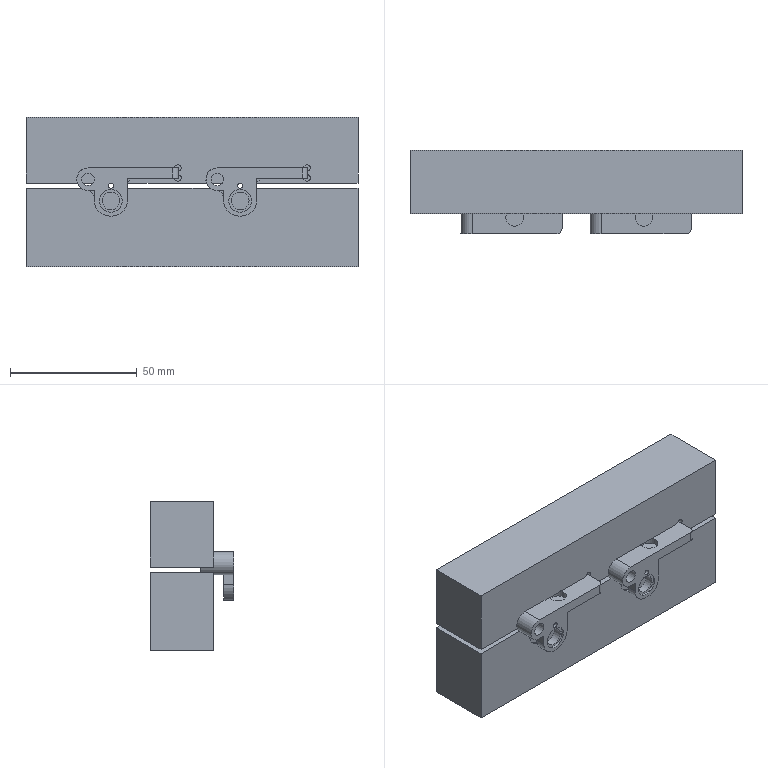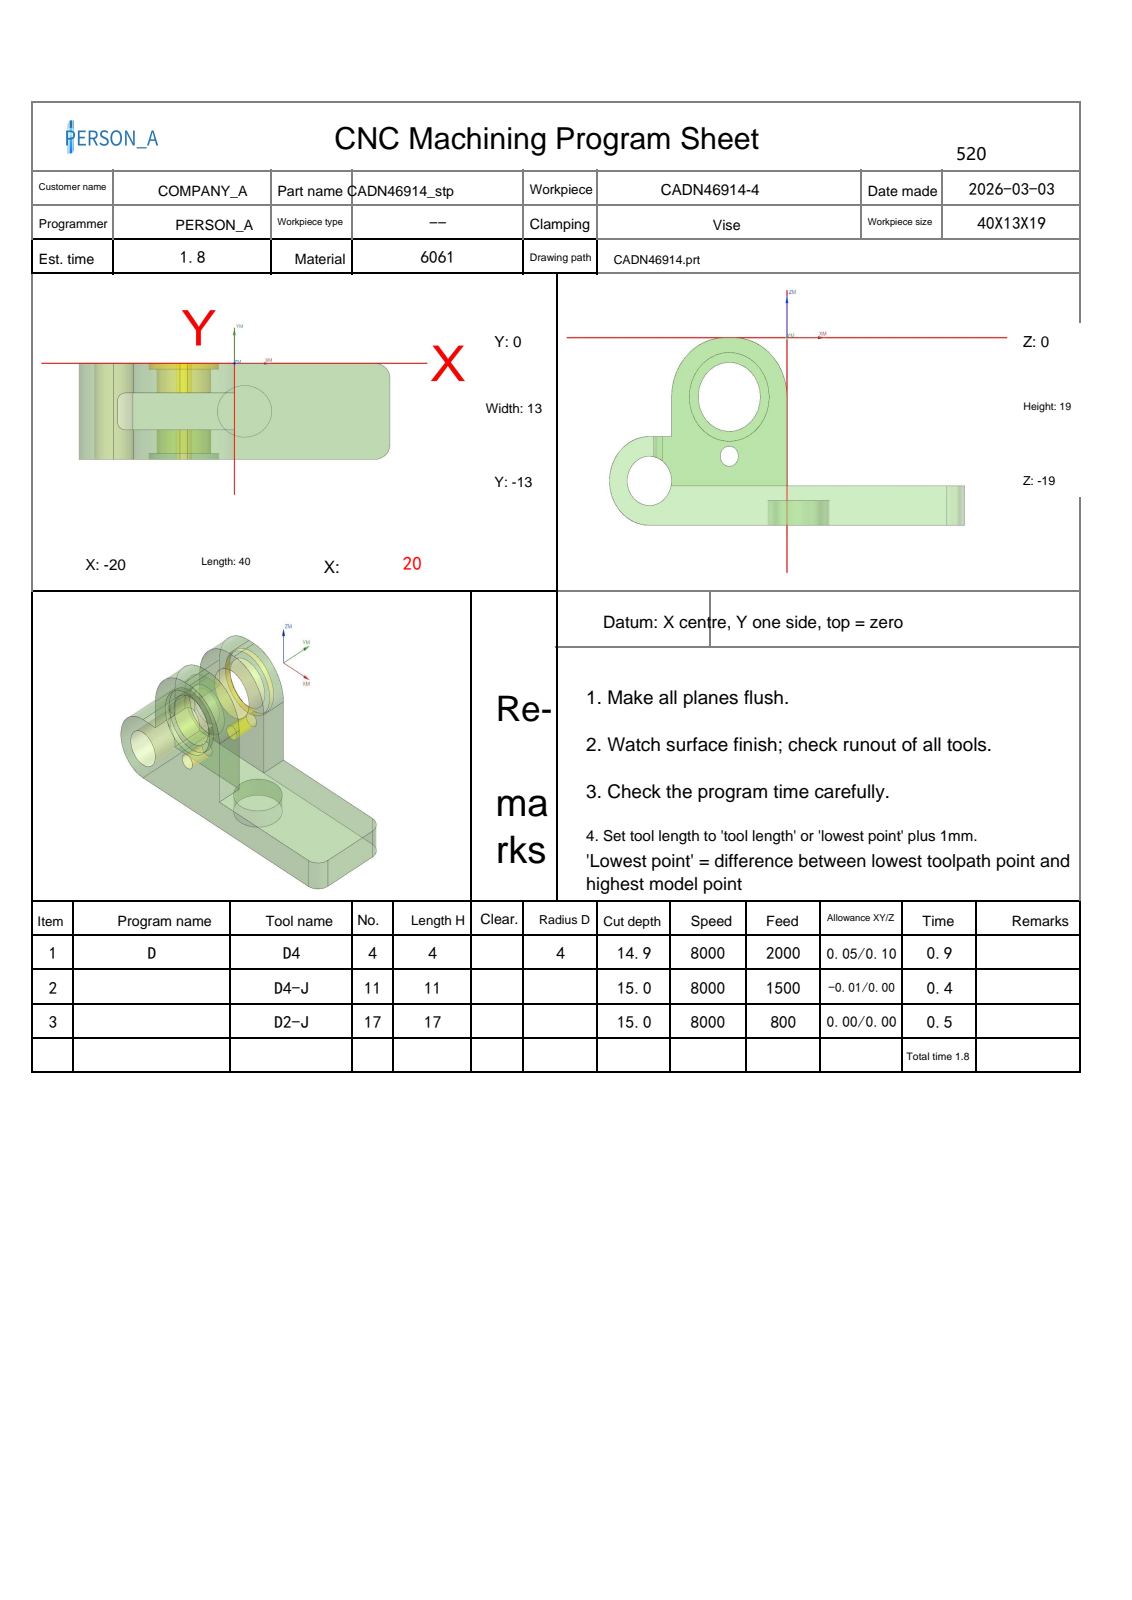NC program | NX | posted by the shop | part box 131 x 33 x 59 mm
Lines 813 to 1839 of 3020:
N3 T17 M06
(D2-J  D=2. R=0. H=17 ce=0.00 di=0.00)
G00 G90 G54 X-12.651 Y-5.2 M03 S8000
G43 H17 Z50.
M08
Z-9.9
G01 X-12.652 Y-5.198 Z-9.93 F800.
X-12.653 Y-5.191 Z-9.958
X-12.656 Y-5.18 Z-9.982
X-12.661 Y-5.165 Z-10.004
X-12.667 Y-5.149 Z-10.023
X-12.675 Y-5.13 Z-10.04
X-12.685 Y-5.11 Z-10.054
X-12.697 Y-5.09 Z-10.066
X-12.711 Y-5.071 Z-10.076
X-12.728 Y-5.052 Z-10.084
X-12.747 Y-5.035 Z-10.09
X-12.769 Y-5.021 Z-10.095
X-12.793 Y-5.01 Z-10.098
X-12.821 Y-5.003 Z-10.099
X-12.851 Y-5. Z-10.1
X-14.
Y-6.149
X-13.989 Y-6.178
X-13.958 Y-6.19
X-13.91 Y-6.188
X-13.849 Y-6.174
X-13.777 Y-6.147 Z-10.101
X-13.699 Y-6.111 Z-10.102
X-13.616 Y-6.067 Z-10.105
X-13.534 Y-6.017 Z-10.108
X-13.325 Y-5.859 Z-10.122
X-13.141 Y-5.673 Z-10.141
X-12.984 Y-5.464 Z-10.162
X-12.934 Y-5.381 Z-10.17
X-12.89 Y-5.299 Z-10.177
X-12.854 Y-5.221 Z-10.183
X-12.827 Y-5.15 Z-10.189
X-12.812 Y-5.089 Z-10.193
X-12.81 Y-5.042 Z-10.197
X-12.822 Y-5.011 Z-10.199
X-12.851 Y-5. Z-10.2
X-13.99
X-14.
Y-6.149
X-13.989 Y-6.178 Z-10.201
X-13.959 Y-6.19 Z-10.202
X-13.911 Y-6.187 Z-10.205
X-13.851 Y-6.172 Z-10.208
X-13.78 Y-6.145 Z-10.212
X-13.703 Y-6.108 Z-10.217
X-13.621 Y-6.064 Z-10.222
X-13.539 Y-6.013 Z-10.227
X-13.331 Y-5.855 Z-10.242
X-13.145 Y-5.669 Z-10.258
X-12.987 Y-5.461 Z-10.273
X-12.936 Y-5.379 Z-10.278
X-12.892 Y-5.298 Z-10.283
X-12.855 Y-5.22 Z-10.288
X-12.828 Y-5.149 Z-10.292
X-12.813 Y-5.089 Z-10.295
X-12.81 Y-5.041 Z-10.298
X-12.822 Y-5.011 Z-10.299
X-12.851 Y-5. Z-10.3
X-13.99
X-14.
Y-6.149
X-13.989 Y-6.178 Z-10.301
X-13.959 Y-6.19 Z-10.302
X-13.911 Y-6.187 Z-10.305
X-13.851 Y-6.172 Z-10.308
X-13.78 Y-6.145 Z-10.312
X-13.703 Y-6.108 Z-10.317
X-13.621 Y-6.064 Z-10.322
X-13.539 Y-6.013 Z-10.327
X-13.331 Y-5.855 Z-10.342
X-13.145 Y-5.669 Z-10.358
X-12.987 Y-5.461 Z-10.373
X-12.936 Y-5.379 Z-10.378
X-12.892 Y-5.298 Z-10.383
X-12.855 Y-5.22 Z-10.388
X-12.828 Y-5.149 Z-10.392
X-12.813 Y-5.089 Z-10.395
X-12.81 Y-5.041 Z-10.398
X-12.822 Y-5.011 Z-10.399
X-12.851 Y-5. Z-10.4
X-13.99
X-14.
Y-6.149
X-13.989 Y-6.178 Z-10.401
X-13.959 Y-6.19 Z-10.402
X-13.911 Y-6.187 Z-10.405
X-13.851 Y-6.172 Z-10.408
X-13.78 Y-6.145 Z-10.412
X-13.703 Y-6.108 Z-10.417
X-13.621 Y-6.064 Z-10.422
X-13.539 Y-6.013 Z-10.427
X-13.331 Y-5.855 Z-10.442
X-13.145 Y-5.669 Z-10.458
X-12.987 Y-5.461 Z-10.473
X-12.936 Y-5.379 Z-10.478
X-12.892 Y-5.298 Z-10.483
X-12.855 Y-5.22 Z-10.488
X-12.828 Y-5.149 Z-10.492
X-12.813 Y-5.089 Z-10.495
X-12.81 Y-5.041 Z-10.498
X-12.822 Y-5.011 Z-10.499
X-12.851 Y-5. Z-10.5
X-13.99
X-14.
Y-6.149
X-13.989 Y-6.178 Z-10.501
X-13.959 Y-6.19 Z-10.502
X-13.911 Y-6.187 Z-10.505
X-13.851 Y-6.172 Z-10.508
X-13.78 Y-6.145 Z-10.512
X-13.703 Y-6.108 Z-10.517
X-13.621 Y-6.064 Z-10.522
X-13.539 Y-6.013 Z-10.527
X-13.331 Y-5.855 Z-10.542
X-13.145 Y-5.669 Z-10.558
X-12.987 Y-5.461 Z-10.573
X-12.936 Y-5.379 Z-10.578
X-12.892 Y-5.298 Z-10.583
X-12.855 Y-5.22 Z-10.588
X-12.828 Y-5.149 Z-10.592
X-12.813 Y-5.089 Z-10.595
X-12.81 Y-5.041 Z-10.598
X-12.822 Y-5.011 Z-10.599
X-12.851 Y-5. Z-10.6
X-13.99
X-14.
Y-6.149
X-13.989 Y-6.178 Z-10.601
X-13.959 Y-6.19 Z-10.602
X-13.911 Y-6.187 Z-10.605
X-13.851 Y-6.172 Z-10.608
X-13.78 Y-6.145 Z-10.612
X-13.703 Y-6.108 Z-10.617
X-13.621 Y-6.064 Z-10.622
X-13.539 Y-6.013 Z-10.627
X-13.331 Y-5.855 Z-10.642
X-13.145 Y-5.669 Z-10.658
X-12.987 Y-5.461 Z-10.673
X-12.936 Y-5.379 Z-10.678
X-12.892 Y-5.298 Z-10.683
X-12.855 Y-5.22 Z-10.688
X-12.828 Y-5.149 Z-10.692
X-12.813 Y-5.089 Z-10.695
X-12.81 Y-5.041 Z-10.698
X-12.822 Y-5.011 Z-10.699
X-12.851 Y-5. Z-10.7
X-13.99
X-14.
Y-6.149
X-13.989 Y-6.178 Z-10.701
X-13.959 Y-6.19 Z-10.702
X-13.911 Y-6.187 Z-10.705
X-13.851 Y-6.172 Z-10.708
X-13.78 Y-6.145 Z-10.712
X-13.703 Y-6.108 Z-10.717
X-13.621 Y-6.064 Z-10.722
X-13.539 Y-6.013 Z-10.727
X-13.331 Y-5.855 Z-10.742
X-13.145 Y-5.669 Z-10.758
X-12.987 Y-5.461 Z-10.773
X-12.936 Y-5.379 Z-10.778
X-12.892 Y-5.298 Z-10.783
X-12.855 Y-5.22 Z-10.788
X-12.828 Y-5.149 Z-10.792
X-12.813 Y-5.089 Z-10.795
X-12.81 Y-5.041 Z-10.798
X-12.822 Y-5.011 Z-10.799
X-12.851 Y-5. Z-10.8
X-13.99
X-14.
Y-6.149
X-13.989 Y-6.178 Z-10.801
X-13.959 Y-6.19 Z-10.802
X-13.911 Y-6.187 Z-10.805
X-13.851 Y-6.172 Z-10.808
X-13.78 Y-6.145 Z-10.812
X-13.703 Y-6.108 Z-10.817
X-13.621 Y-6.064 Z-10.822
X-13.539 Y-6.013 Z-10.827
X-13.331 Y-5.855 Z-10.842
X-13.145 Y-5.669 Z-10.858
X-12.987 Y-5.461 Z-10.873
X-12.936 Y-5.379 Z-10.878
X-12.892 Y-5.298 Z-10.883
X-12.855 Y-5.22 Z-10.888
X-12.828 Y-5.149 Z-10.892
X-12.813 Y-5.089 Z-10.895
X-12.81 Y-5.041 Z-10.898
X-12.822 Y-5.011 Z-10.899
X-12.851 Y-5. Z-10.9
X-13.99
X-14.
Y-6.149
X-13.989 Y-6.178 Z-10.901
X-13.959 Y-6.19 Z-10.902
X-13.911 Y-6.187 Z-10.905
X-13.851 Y-6.172 Z-10.908
X-13.78 Y-6.145 Z-10.912
X-13.703 Y-6.108 Z-10.917
X-13.621 Y-6.064 Z-10.922
X-13.539 Y-6.013 Z-10.927
X-13.331 Y-5.855 Z-10.942
X-13.145 Y-5.669 Z-10.958
X-12.987 Y-5.461 Z-10.973
X-12.936 Y-5.379 Z-10.978
X-12.892 Y-5.298 Z-10.983
X-12.855 Y-5.22 Z-10.988
X-12.828 Y-5.149 Z-10.992
X-12.813 Y-5.089 Z-10.995
X-12.81 Y-5.041 Z-10.998
X-12.822 Y-5.011 Z-10.999
X-12.851 Y-5. Z-11.
X-13.99
X-14.
Y-6.149
X-13.989 Y-6.178 Z-11.001
X-13.959 Y-6.19 Z-11.002
X-13.911 Y-6.187 Z-11.005
X-13.851 Y-6.172 Z-11.008
X-13.78 Y-6.145 Z-11.012
X-13.703 Y-6.108 Z-11.017
X-13.621 Y-6.064 Z-11.022
X-13.539 Y-6.013 Z-11.027
X-13.331 Y-5.855 Z-11.042
X-13.145 Y-5.669 Z-11.058
X-12.987 Y-5.461 Z-11.073
X-12.936 Y-5.379 Z-11.078
X-12.892 Y-5.298 Z-11.083
X-12.855 Y-5.22 Z-11.088
X-12.828 Y-5.149 Z-11.092
X-12.813 Y-5.089 Z-11.095
X-12.81 Y-5.041 Z-11.098
X-12.822 Y-5.011 Z-11.099
X-12.851 Y-5. Z-11.1
X-13.99
X-14.
Y-6.149
X-13.989 Y-6.178 Z-11.101
X-13.959 Y-6.19 Z-11.102
X-13.911 Y-6.187 Z-11.105
X-13.851 Y-6.172 Z-11.108
X-13.78 Y-6.145 Z-11.112
X-13.703 Y-6.108 Z-11.117
X-13.621 Y-6.064 Z-11.122
X-13.539 Y-6.013 Z-11.127
X-13.331 Y-5.855 Z-11.142
X-13.145 Y-5.669 Z-11.158
X-12.987 Y-5.461 Z-11.173
X-12.936 Y-5.379 Z-11.178
X-12.892 Y-5.298 Z-11.183
X-12.855 Y-5.22 Z-11.188
X-12.828 Y-5.149 Z-11.192
X-12.813 Y-5.089 Z-11.195
X-12.81 Y-5.041 Z-11.198
X-12.822 Y-5.011 Z-11.199
X-12.851 Y-5. Z-11.2
X-13.99
X-14.
Y-6.149
X-13.989 Y-6.178 Z-11.201
X-13.959 Y-6.19 Z-11.202
X-13.911 Y-6.187 Z-11.205
X-13.851 Y-6.172 Z-11.208
X-13.78 Y-6.145 Z-11.212
X-13.703 Y-6.108 Z-11.217
X-13.621 Y-6.064 Z-11.222
X-13.539 Y-6.013 Z-11.227
X-13.331 Y-5.855 Z-11.242
X-13.145 Y-5.669 Z-11.258
X-12.987 Y-5.461 Z-11.273
X-12.936 Y-5.379 Z-11.278
X-12.892 Y-5.298 Z-11.283
X-12.855 Y-5.22 Z-11.288
X-12.828 Y-5.149 Z-11.292
X-12.813 Y-5.089 Z-11.295
X-12.81 Y-5.041 Z-11.298
X-12.822 Y-5.011 Z-11.299
X-12.851 Y-5. Z-11.3
X-13.99
X-14.
Y-6.149
X-13.989 Y-6.178 Z-11.301
X-13.959 Y-6.19 Z-11.302
X-13.911 Y-6.187 Z-11.305
X-13.851 Y-6.172 Z-11.308
X-13.78 Y-6.145 Z-11.312
X-13.703 Y-6.108 Z-11.317
X-13.621 Y-6.064 Z-11.322
X-13.539 Y-6.013 Z-11.327
X-13.331 Y-5.855 Z-11.342
X-13.145 Y-5.669 Z-11.358
X-12.987 Y-5.461 Z-11.373
X-12.936 Y-5.379 Z-11.378
X-12.892 Y-5.298 Z-11.383
X-12.855 Y-5.22 Z-11.388
X-12.828 Y-5.149 Z-11.392
X-12.813 Y-5.089 Z-11.395
X-12.81 Y-5.041 Z-11.398
X-12.822 Y-5.011 Z-11.399
X-12.851 Y-5. Z-11.4
X-13.99
X-14.
Y-6.149
X-13.989 Y-6.178 Z-11.401
X-13.959 Y-6.19 Z-11.402
X-13.911 Y-6.187 Z-11.405
X-13.851 Y-6.172 Z-11.408
X-13.78 Y-6.145 Z-11.412
X-13.703 Y-6.108 Z-11.417
X-13.621 Y-6.064 Z-11.422
X-13.539 Y-6.013 Z-11.427
X-13.331 Y-5.855 Z-11.442
X-13.145 Y-5.669 Z-11.458
X-12.987 Y-5.461 Z-11.473
X-12.936 Y-5.379 Z-11.478
X-12.892 Y-5.298 Z-11.483
X-12.855 Y-5.22 Z-11.488
X-12.828 Y-5.149 Z-11.492
X-12.813 Y-5.089 Z-11.495
X-12.81 Y-5.041 Z-11.498
X-12.822 Y-5.011 Z-11.499
X-12.851 Y-5. Z-11.5
X-13.99
X-14.
Y-6.149
X-13.989 Y-6.178 Z-11.501
X-13.959 Y-6.19 Z-11.502
X-13.911 Y-6.187 Z-11.505
X-13.851 Y-6.172 Z-11.508
X-13.78 Y-6.145 Z-11.512
X-13.703 Y-6.108 Z-11.517
X-13.621 Y-6.064 Z-11.522
X-13.539 Y-6.013 Z-11.527
X-13.331 Y-5.855 Z-11.542
X-13.145 Y-5.669 Z-11.558
X-12.987 Y-5.461 Z-11.573
X-12.936 Y-5.379 Z-11.578
X-12.892 Y-5.298 Z-11.583
X-12.855 Y-5.22 Z-11.588
X-12.828 Y-5.149 Z-11.592
X-12.813 Y-5.089 Z-11.595
X-12.81 Y-5.041 Z-11.598
X-12.822 Y-5.011 Z-11.599
X-12.851 Y-5. Z-11.6
X-13.99
X-14.
Y-6.149
X-13.989 Y-6.178 Z-11.601
X-13.959 Y-6.19 Z-11.602
X-13.911 Y-6.187 Z-11.605
X-13.851 Y-6.172 Z-11.608
X-13.78 Y-6.145 Z-11.612
X-13.703 Y-6.108 Z-11.617
X-13.621 Y-6.064 Z-11.622
X-13.539 Y-6.013 Z-11.627
X-13.331 Y-5.855 Z-11.642
X-13.145 Y-5.669 Z-11.658
X-12.987 Y-5.461 Z-11.673
X-12.936 Y-5.379 Z-11.678
X-12.892 Y-5.298 Z-11.683
X-12.855 Y-5.22 Z-11.688
X-12.828 Y-5.149 Z-11.692
X-12.813 Y-5.089 Z-11.695
X-12.81 Y-5.041 Z-11.698
X-12.822 Y-5.011 Z-11.699
X-12.851 Y-5. Z-11.7
X-13.99
X-14.
Y-6.149
X-13.989 Y-6.178 Z-11.701
X-13.959 Y-6.19 Z-11.702
X-13.911 Y-6.187 Z-11.705
X-13.851 Y-6.172 Z-11.708
X-13.78 Y-6.145 Z-11.712
X-13.703 Y-6.108 Z-11.717
X-13.621 Y-6.064 Z-11.722
X-13.539 Y-6.013 Z-11.727
X-13.331 Y-5.855 Z-11.742
X-13.145 Y-5.669 Z-11.758
X-12.987 Y-5.461 Z-11.773
X-12.936 Y-5.379 Z-11.778
X-12.892 Y-5.298 Z-11.783
X-12.855 Y-5.22 Z-11.788
X-12.828 Y-5.149 Z-11.792
X-12.813 Y-5.089 Z-11.795
X-12.81 Y-5.041 Z-11.798
X-12.822 Y-5.011 Z-11.799
X-12.851 Y-5. Z-11.8
X-13.99
X-14.
Y-6.149
X-13.989 Y-6.178 Z-11.801
X-13.959 Y-6.19 Z-11.802
X-13.911 Y-6.187 Z-11.805
X-13.851 Y-6.172 Z-11.808
X-13.78 Y-6.145 Z-11.812
X-13.703 Y-6.108 Z-11.817
X-13.621 Y-6.064 Z-11.822
X-13.539 Y-6.013 Z-11.827
X-13.331 Y-5.855 Z-11.842
X-13.145 Y-5.669 Z-11.858
X-12.987 Y-5.461 Z-11.873
X-12.936 Y-5.379 Z-11.878
X-12.892 Y-5.298 Z-11.883
X-12.855 Y-5.22 Z-11.888
X-12.828 Y-5.149 Z-11.892
X-12.813 Y-5.089 Z-11.895
X-12.81 Y-5.041 Z-11.898
X-12.822 Y-5.011 Z-11.899
X-12.851 Y-5. Z-11.9
X-13.99
X-14.
Y-6.149
X-13.989 Y-6.178 Z-11.901
X-13.959 Y-6.19 Z-11.902
X-13.911 Y-6.187 Z-11.905
X-13.851 Y-6.172 Z-11.908
X-13.78 Y-6.145 Z-11.912
X-13.703 Y-6.108 Z-11.917
X-13.621 Y-6.064 Z-11.922
X-13.539 Y-6.013 Z-11.927
X-13.331 Y-5.855 Z-11.942
X-13.145 Y-5.669 Z-11.958
X-12.987 Y-5.461 Z-11.973
X-12.936 Y-5.379 Z-11.978
X-12.892 Y-5.298 Z-11.983
X-12.855 Y-5.22 Z-11.988
X-12.828 Y-5.149 Z-11.992
X-12.813 Y-5.089 Z-11.995
X-12.81 Y-5.041 Z-11.998
X-12.822 Y-5.011 Z-11.999
X-12.851 Y-5. Z-12.
X-13.99
X-14.
Y-6.149
X-13.989 Y-6.178 Z-12.001
X-13.959 Y-6.19 Z-12.002
X-13.911 Y-6.187 Z-12.005
X-13.851 Y-6.172 Z-12.008
X-13.78 Y-6.145 Z-12.012
X-13.703 Y-6.108 Z-12.017
X-13.621 Y-6.064 Z-12.022
X-13.539 Y-6.013 Z-12.027
X-13.331 Y-5.855 Z-12.042
X-13.145 Y-5.669 Z-12.058
X-12.987 Y-5.461 Z-12.073
X-12.936 Y-5.379 Z-12.078
X-12.892 Y-5.298 Z-12.083
X-12.855 Y-5.22 Z-12.088
X-12.828 Y-5.149 Z-12.092
X-12.813 Y-5.089 Z-12.095
X-12.81 Y-5.041 Z-12.098
X-12.822 Y-5.011 Z-12.099
X-12.851 Y-5. Z-12.1
X-14.
Y-6.149
X-13.989 Y-6.179 Z-12.101
X-13.958 Y-6.194 Z-12.102
X-13.91 Y-6.196 Z-12.105
X-13.848 Y-6.186 Z-12.108
X-13.777 Y-6.165 Z-12.112
X-13.698 Y-6.134 Z-12.117
X-13.615 Y-6.094 Z-12.122
X-13.533 Y-6.046 Z-12.127
X-13.374 Y-5.933 Z-12.138
X-13.229 Y-5.798 Z-12.15
X-13.098 Y-5.646 Z-12.162
X-12.984 Y-5.48 Z-12.173
X-12.933 Y-5.394 Z-12.178
X-12.89 Y-5.309 Z-12.183
X-12.853 Y-5.228 Z-12.188
X-12.827 Y-5.155 Z-12.192
X-12.812 Y-5.092 Z-12.195
X-12.81 Y-5.043 Z-12.198
X-12.822 Y-5.011 Z-12.199
X-12.851 Y-5. Z-12.2
X-14.
Y-6.149
X-13.989 Y-6.18 Z-12.201
X-13.958 Y-6.197 Z-12.202
X-13.911 Y-6.202 Z-12.205
X-13.85 Y-6.195 Z-12.208
X-13.779 Y-6.177 Z-12.212
X-13.701 Y-6.15 Z-12.217
X-13.619 Y-6.113 Z-12.222
X-13.536 Y-6.068 Z-12.227
X-13.378 Y-5.956 Z-12.238
X-13.233 Y-5.819 Z-12.25
X-13.101 Y-5.663 Z-12.262
X-12.986 Y-5.492 Z-12.273
X-12.935 Y-5.404 Z-12.278
X-12.891 Y-5.317 Z-12.283
X-12.854 Y-5.234 Z-12.288
X-12.828 Y-5.158 Z-12.292
X-12.812 Y-5.094 Z-12.295
X-12.81 Y-5.044 Z-12.298
X-12.822 Y-5.012 Z-12.299
X-12.851 Y-5. Z-12.3
X-14.
Y-6.149
X-13.986 Y-6.184 Z-12.301
X-13.948 Y-6.202 Z-12.303
X-13.89 Y-6.206 Z-12.306
X-13.816 Y-6.195 Z-12.31
X-13.731 Y-6.171 Z-12.315
X-13.64 Y-6.134 Z-12.321
X-13.547 Y-6.085 Z-12.327
X-13.39 Y-5.974 Z-12.338
X-13.243 Y-5.836 Z-12.35
X-13.11 Y-5.676 Z-12.362
X-12.992 Y-5.502 Z-12.373
X-12.94 Y-5.412 Z-12.378
X-12.895 Y-5.323 Z-12.383
X-12.857 Y-5.238 Z-12.388
X-12.83 Y-5.161 Z-12.392
X-12.813 Y-5.096 Z-12.395
X-12.81 Y-5.045 Z-12.398
X-12.822 Y-5.012 Z-12.399
X-12.851 Y-5. Z-12.4
X-14.
Y-6.149
X-13.988 Y-6.184 Z-12.401
X-13.953 Y-6.203 Z-12.403
X-13.9 Y-6.208 Z-12.406
X-13.832 Y-6.198 Z-12.41
X-13.754 Y-6.175 Z-12.415
X-13.668 Y-6.139 Z-12.421
X-13.579 Y-6.091 Z-12.427
X-13.423 Y-5.981 Z-12.438
X-13.273 Y-5.842 Z-12.449
X-13.133 Y-5.681 Z-12.461
X-13.008 Y-5.506 Z-12.472
X-12.953 Y-5.415 Z-12.477
X-12.904 Y-5.325 Z-12.483
X-12.864 Y-5.24 Z-12.487
X-12.834 Y-5.162 Z-12.492
X-12.816 Y-5.096 Z-12.495
X-12.812 Y-5.045 Z-12.498
X-12.823 Y-5.012 Z-12.499
X-12.851 Y-5. Z-12.5
X-14.
Y-6.149
X-13.988 Y-6.184 Z-12.501
X-13.953 Y-6.203 Z-12.503
X-13.9 Y-6.208 Z-12.506
X-13.832 Y-6.199 Z-12.51
X-13.754 Y-6.176 Z-12.515
X-13.668 Y-6.14 Z-12.52
X-13.579 Y-6.092 Z-12.526
X-13.424 Y-5.982 Z-12.538
X-13.274 Y-5.843 Z-12.549
X-13.135 Y-5.682 Z-12.561
X-13.01 Y-5.506 Z-12.573
X-12.954 Y-5.415 Z-12.578
X-12.906 Y-5.325 Z-12.583
X-12.865 Y-5.24 Z-12.588
X-12.835 Y-5.162 Z-12.592
X-12.816 Y-5.096 Z-12.595
X-12.812 Y-5.045 Z-12.598
X-12.823 Y-5.012 Z-12.599
X-12.851 Y-5. Z-12.6
X-14.
Y-6.149
X-13.988 Y-6.184 Z-12.601
X-13.953 Y-6.203 Z-12.603
X-13.9 Y-6.208 Z-12.606
X-13.833 Y-6.198 Z-12.61
X-13.754 Y-6.175 Z-12.615
X-13.669 Y-6.139 Z-12.621
X-13.58 Y-6.092 Z-12.627
X-13.425 Y-5.981 Z-12.638
X-13.275 Y-5.842 Z-12.65
X-13.135 Y-5.682 Z-12.662
X-13.01 Y-5.506 Z-12.673
X-12.955 Y-5.415 Z-12.678
X-12.906 Y-5.325 Z-12.683
X-12.865 Y-5.24 Z-12.688
X-12.835 Y-5.162 Z-12.692
X-12.817 Y-5.096 Z-12.695
X-12.812 Y-5.045 Z-12.698
X-12.823 Y-5.012 Z-12.699
X-12.851 Y-5. Z-12.7
X-14.
Y-6.149
X-13.988 Y-6.184 Z-12.701
X-13.953 Y-6.203 Z-12.703
X-13.9 Y-6.208 Z-12.706
X-13.833 Y-6.198 Z-12.71
X-13.754 Y-6.175 Z-12.715
X-13.669 Y-6.139 Z-12.721
X-13.58 Y-6.092 Z-12.727
X-13.425 Y-5.981 Z-12.738
X-13.275 Y-5.842 Z-12.75
X-13.135 Y-5.682 Z-12.762
X-13.01 Y-5.506 Z-12.773
X-12.955 Y-5.415 Z-12.778
X-12.906 Y-5.325 Z-12.783
X-12.865 Y-5.24 Z-12.788
X-12.835 Y-5.162 Z-12.792
X-12.817 Y-5.096 Z-12.795
X-12.812 Y-5.045 Z-12.798
X-12.823 Y-5.012 Z-12.799
X-12.851 Y-5. Z-12.8
X-14.
Y-6.149
X-13.988 Y-6.184 Z-12.801
X-13.953 Y-6.203 Z-12.803
X-13.9 Y-6.208 Z-12.806
X-13.833 Y-6.198 Z-12.81
X-13.754 Y-6.175 Z-12.815
X-13.669 Y-6.139 Z-12.821
X-13.58 Y-6.092 Z-12.827
X-13.425 Y-5.981 Z-12.838
X-13.275 Y-5.842 Z-12.85
X-13.135 Y-5.682 Z-12.862
X-13.01 Y-5.506 Z-12.873
X-12.955 Y-5.415 Z-12.878
X-12.906 Y-5.325 Z-12.883
X-12.865 Y-5.24 Z-12.888
X-12.835 Y-5.162 Z-12.892
X-12.817 Y-5.096 Z-12.895
X-12.812 Y-5.045 Z-12.898
X-12.823 Y-5.012 Z-12.899
X-12.851 Y-5. Z-12.9
X-14.
Y-6.149
X-13.988 Y-6.184 Z-12.901
X-13.953 Y-6.203 Z-12.903
X-13.9 Y-6.208 Z-12.906
X-13.833 Y-6.198 Z-12.91
X-13.754 Y-6.175 Z-12.915
X-13.669 Y-6.139 Z-12.921
X-13.58 Y-6.092 Z-12.927
X-13.425 Y-5.981 Z-12.938
X-13.275 Y-5.842 Z-12.95
X-13.135 Y-5.682 Z-12.962
X-13.01 Y-5.506 Z-12.973
X-12.955 Y-5.415 Z-12.978
X-12.906 Y-5.325 Z-12.983
X-12.865 Y-5.24 Z-12.988
X-12.835 Y-5.162 Z-12.992
X-12.817 Y-5.096 Z-12.995
X-12.812 Y-5.045 Z-12.998
X-12.823 Y-5.012 Z-12.999
X-12.851 Y-5. Z-13.
X-14.
Y-6.149
X-13.988 Y-6.184 Z-13.001
X-13.953 Y-6.203 Z-13.003
X-13.9 Y-6.208 Z-13.006
X-13.833 Y-6.198 Z-13.01
X-13.754 Y-6.175 Z-13.015
X-13.669 Y-6.139 Z-13.021
X-13.58 Y-6.092 Z-13.027
X-13.425 Y-5.981 Z-13.038
X-13.275 Y-5.842 Z-13.05
X-13.135 Y-5.682 Z-13.062
X-13.01 Y-5.506 Z-13.073
X-12.955 Y-5.415 Z-13.078
X-12.906 Y-5.325 Z-13.083
X-12.865 Y-5.24 Z-13.088
X-12.835 Y-5.162 Z-13.092
X-12.817 Y-5.096 Z-13.095
X-12.812 Y-5.045 Z-13.098
X-12.823 Y-5.012 Z-13.099
X-12.851 Y-5. Z-13.1
X-14.
Y-6.149
X-13.988 Y-6.184 Z-13.101
X-13.953 Y-6.203 Z-13.103
X-13.9 Y-6.208 Z-13.106
X-13.833 Y-6.198 Z-13.11
X-13.754 Y-6.175 Z-13.115
X-13.669 Y-6.139 Z-13.121
X-13.58 Y-6.092 Z-13.127
X-13.425 Y-5.981 Z-13.138
X-13.275 Y-5.842 Z-13.15
X-13.135 Y-5.682 Z-13.162
X-13.01 Y-5.506 Z-13.173
X-12.955 Y-5.415 Z-13.178
X-12.906 Y-5.325 Z-13.183
X-12.865 Y-5.24 Z-13.188
X-12.835 Y-5.162 Z-13.192
X-12.817 Y-5.096 Z-13.195
X-12.812 Y-5.045 Z-13.198
X-12.823 Y-5.012 Z-13.199
X-12.851 Y-5. Z-13.2
X-14.
Y-6.149
X-13.988 Y-6.184 Z-13.201
X-13.953 Y-6.203 Z-13.203
X-13.9 Y-6.208 Z-13.206
X-13.833 Y-6.198 Z-13.21
X-13.754 Y-6.175 Z-13.215
X-13.669 Y-6.139 Z-13.221
X-13.58 Y-6.092 Z-13.227
X-13.425 Y-5.981 Z-13.238
X-13.275 Y-5.842 Z-13.25
X-13.135 Y-5.682 Z-13.262
X-13.01 Y-5.506 Z-13.273
X-12.955 Y-5.415 Z-13.278
X-12.906 Y-5.325 Z-13.283
X-12.865 Y-5.24 Z-13.288
X-12.835 Y-5.162 Z-13.292
X-12.817 Y-5.096 Z-13.295
X-12.812 Y-5.045 Z-13.298
X-12.823 Y-5.012 Z-13.299
X-12.851 Y-5. Z-13.3
X-14.
Y-6.149
X-13.988 Y-6.184 Z-13.301
X-13.953 Y-6.203 Z-13.303
X-13.9 Y-6.208 Z-13.306
X-13.833 Y-6.198 Z-13.31
X-13.754 Y-6.175 Z-13.315
X-13.669 Y-6.139 Z-13.321
X-13.58 Y-6.092 Z-13.327
X-13.425 Y-5.981 Z-13.338
X-13.275 Y-5.842 Z-13.35
X-13.135 Y-5.682 Z-13.362
X-13.01 Y-5.506 Z-13.373
X-12.955 Y-5.415 Z-13.378
X-12.906 Y-5.325 Z-13.383
X-12.865 Y-5.24 Z-13.388
X-12.835 Y-5.162 Z-13.392
X-12.817 Y-5.096 Z-13.395
X-12.812 Y-5.045 Z-13.398
X-12.823 Y-5.012 Z-13.399
X-12.851 Y-5. Z-13.4
X-14.
Y-6.149
X-13.988 Y-6.184 Z-13.401
X-13.953 Y-6.203 Z-13.403
X-13.9 Y-6.208 Z-13.406
X-13.833 Y-6.198 Z-13.41
X-13.754 Y-6.175 Z-13.415
X-13.669 Y-6.139 Z-13.421
X-13.58 Y-6.092 Z-13.427
X-13.425 Y-5.981 Z-13.438
X-13.275 Y-5.842 Z-13.45
X-13.135 Y-5.682 Z-13.462
X-13.01 Y-5.506 Z-13.473
X-12.955 Y-5.415 Z-13.478
X-12.906 Y-5.325 Z-13.483
X-12.865 Y-5.24 Z-13.488
X-12.835 Y-5.162 Z-13.492
X-12.817 Y-5.096 Z-13.495
X-12.812 Y-5.045 Z-13.498
X-12.823 Y-5.012 Z-13.499
X-12.851 Y-5. Z-13.5
X-14.
Y-6.149
X-13.988 Y-6.184 Z-13.501
X-13.953 Y-6.203 Z-13.503
X-13.9 Y-6.208 Z-13.506
X-13.833 Y-6.198 Z-13.51
X-13.754 Y-6.175 Z-13.515
X-13.669 Y-6.139 Z-13.521
X-13.58 Y-6.092 Z-13.527
X-13.425 Y-5.981 Z-13.538
X-13.275 Y-5.842 Z-13.55
X-13.135 Y-5.682 Z-13.562
X-13.01 Y-5.506 Z-13.573
X-12.955 Y-5.415 Z-13.578
X-12.906 Y-5.325 Z-13.583
X-12.865 Y-5.24 Z-13.588
X-12.835 Y-5.162 Z-13.592
X-12.817 Y-5.096 Z-13.595
X-12.812 Y-5.045 Z-13.598
X-12.823 Y-5.012 Z-13.599
X-12.851 Y-5. Z-13.6
X-14.
Y-6.149
X-13.988 Y-6.184 Z-13.601
X-13.953 Y-6.203 Z-13.603
X-13.9 Y-6.208 Z-13.606
X-13.833 Y-6.198 Z-13.61
X-13.754 Y-6.175 Z-13.615
X-13.669 Y-6.139 Z-13.621
X-13.58 Y-6.092 Z-13.627
X-13.425 Y-5.981 Z-13.638
X-13.275 Y-5.842 Z-13.65
X-13.135 Y-5.682 Z-13.662
X-13.01 Y-5.506 Z-13.673
X-12.955 Y-5.415 Z-13.678
X-12.906 Y-5.325 Z-13.683
X-12.865 Y-5.24 Z-13.688
X-12.835 Y-5.162 Z-13.692
X-12.817 Y-5.096 Z-13.695
X-12.812 Y-5.045 Z-13.698
X-12.823 Y-5.012 Z-13.699
X-12.851 Y-5. Z-13.7
X-14.
Y-6.149
X-13.988 Y-6.184 Z-13.701
X-13.953 Y-6.203 Z-13.703
X-13.9 Y-6.208 Z-13.706
X-13.833 Y-6.198 Z-13.71
X-13.754 Y-6.175 Z-13.715
X-13.669 Y-6.139 Z-13.721
X-13.58 Y-6.092 Z-13.727
X-13.425 Y-5.981 Z-13.738
X-13.275 Y-5.842 Z-13.75
X-13.135 Y-5.682 Z-13.762
X-13.01 Y-5.506 Z-13.773
X-12.955 Y-5.415 Z-13.778
X-12.906 Y-5.325 Z-13.783
X-12.865 Y-5.24 Z-13.788
X-12.835 Y-5.162 Z-13.792
X-12.817 Y-5.096 Z-13.795
X-12.812 Y-5.045 Z-13.798
X-12.823 Y-5.012 Z-13.799
X-12.851 Y-5. Z-13.8
X-14.
Y-6.149
X-13.988 Y-6.184 Z-13.801
X-13.953 Y-6.203 Z-13.803
X-13.9 Y-6.208 Z-13.806
X-13.833 Y-6.198 Z-13.81
X-13.754 Y-6.175 Z-13.815
X-13.669 Y-6.139 Z-13.821
X-13.58 Y-6.092 Z-13.827
X-13.425 Y-5.981 Z-13.838
X-13.275 Y-5.842 Z-13.85
X-13.135 Y-5.682 Z-13.862
X-13.01 Y-5.506 Z-13.873
X-12.955 Y-5.415 Z-13.878
X-12.906 Y-5.325 Z-13.883
X-12.865 Y-5.24 Z-13.888
X-12.835 Y-5.162 Z-13.892
X-12.817 Y-5.096 Z-13.895
X-12.812 Y-5.045 Z-13.898
X-12.823 Y-5.012 Z-13.899
X-12.851 Y-5. Z-13.9
X-14.
Y-6.149
X-13.988 Y-6.184 Z-13.901
X-13.953 Y-6.203 Z-13.903
X-13.9 Y-6.208 Z-13.906
X-13.833 Y-6.198 Z-13.91
X-13.754 Y-6.175 Z-13.915
X-13.669 Y-6.139 Z-13.921
X-13.58 Y-6.092 Z-13.927
X-13.425 Y-5.981 Z-13.938
X-13.275 Y-5.842 Z-13.95
X-13.135 Y-5.682 Z-13.962
X-13.01 Y-5.506 Z-13.973
X-12.955 Y-5.415 Z-13.978
X-12.906 Y-5.325 Z-13.983
X-12.865 Y-5.24 Z-13.988
X-12.835 Y-5.162 Z-13.992
X-12.817 Y-5.096 Z-13.995
X-12.812 Y-5.045 Z-13.998
X-12.823 Y-5.012 Z-13.999
X-12.851 Y-5. Z-14.
X-14.
Y-6.149
X-13.988 Y-6.184 Z-14.001
X-13.953 Y-6.203 Z-14.003
X-13.9 Y-6.208 Z-14.006
X-13.833 Y-6.198 Z-14.01
X-13.754 Y-6.175 Z-14.015
X-13.669 Y-6.139 Z-14.021
X-13.58 Y-6.092 Z-14.027
X-13.425 Y-5.981 Z-14.038
X-13.275 Y-5.842 Z-14.05
X-13.135 Y-5.682 Z-14.062
X-13.01 Y-5.506 Z-14.073
X-12.955 Y-5.415 Z-14.078
X-12.906 Y-5.325 Z-14.083
X-12.865 Y-5.24 Z-14.088
X-12.835 Y-5.162 Z-14.092
X-12.817 Y-5.096 Z-14.095
X-12.812 Y-5.045 Z-14.098
X-12.823 Y-5.012 Z-14.099
X-12.851 Y-5. Z-14.1
X-14.
Y-6.149
X-13.988 Y-6.184 Z-14.101
X-13.953 Y-6.203 Z-14.103
X-13.9 Y-6.208 Z-14.106
X-13.833 Y-6.198 Z-14.11
X-13.754 Y-6.175 Z-14.115
X-13.669 Y-6.139 Z-14.121
X-13.58 Y-6.092 Z-14.127
X-13.425 Y-5.981 Z-14.138
X-13.275 Y-5.842 Z-14.15
X-13.135 Y-5.682 Z-14.162
X-13.01 Y-5.506 Z-14.173
X-12.955 Y-5.415 Z-14.178
X-12.906 Y-5.325 Z-14.183
X-12.865 Y-5.24 Z-14.188
X-12.835 Y-5.162 Z-14.192
X-12.817 Y-5.096 Z-14.195
X-12.812 Y-5.045 Z-14.198
X-12.823 Y-5.012 Z-14.199
X-12.851 Y-5. Z-14.2
X-14.
Y-6.149
X-13.988 Y-6.184 Z-14.201
X-13.953 Y-6.203 Z-14.203
X-13.9 Y-6.208 Z-14.206
X-13.833 Y-6.198 Z-14.21
X-13.754 Y-6.175 Z-14.215
X-13.669 Y-6.139 Z-14.221
X-13.58 Y-6.092 Z-14.227
X-13.425 Y-5.981 Z-14.238
X-13.275 Y-5.842 Z-14.25
X-13.135 Y-5.682 Z-14.262
X-13.01 Y-5.506 Z-14.273
X-12.955 Y-5.415 Z-14.278
X-12.906 Y-5.325 Z-14.283
X-12.865 Y-5.24 Z-14.288
X-12.835 Y-5.162 Z-14.292
X-12.817 Y-5.096 Z-14.295
X-12.812 Y-5.045 Z-14.298
X-12.823 Y-5.012 Z-14.299
X-12.851 Y-5. Z-14.3
X-14.
Y-6.149
X-13.988 Y-6.184 Z-14.301
X-13.953 Y-6.203 Z-14.303
X-13.9 Y-6.208 Z-14.306
X-13.833 Y-6.198 Z-14.31
X-13.754 Y-6.175 Z-14.315
X-13.669 Y-6.139 Z-14.321
X-13.58 Y-6.092 Z-14.327
X-13.425 Y-5.981 Z-14.338
X-13.275 Y-5.842 Z-14.35
X-13.135 Y-5.682 Z-14.362
X-13.01 Y-5.506 Z-14.373
X-12.955 Y-5.415 Z-14.378
X-12.906 Y-5.325 Z-14.383
X-12.865 Y-5.24 Z-14.388
X-12.835 Y-5.162 Z-14.392
X-12.817 Y-5.096 Z-14.395
X-12.812 Y-5.045 Z-14.398
X-12.823 Y-5.012 Z-14.399
X-12.851 Y-5. Z-14.4
X-14.
Y-6.149
X-13.988 Y-6.184 Z-14.401
X-13.953 Y-6.203 Z-14.403
X-13.9 Y-6.208 Z-14.406
X-13.833 Y-6.198 Z-14.41
X-13.754 Y-6.175 Z-14.415
X-13.669 Y-6.139 Z-14.421
X-13.58 Y-6.091 Z-14.427
X-13.425 Y-5.981 Z-14.438
X-13.275 Y-5.842 Z-14.45
X-13.135 Y-5.682 Z-14.462
X-13.01 Y-5.506 Z-14.473
X-12.955 Y-5.415 Z-14.478
X-12.906 Y-5.325 Z-14.483
X-12.865 Y-5.24 Z-14.488
X-12.835 Y-5.162 Z-14.492
X-12.817 Y-5.096 Z-14.495
X-12.812 Y-5.045 Z-14.498
X-12.823 Y-5.012 Z-14.499
X-12.851 Y-5. Z-14.5
X-14.
Y-6.149
X-13.988 Y-6.184 Z-14.501
X-13.953 Y-6.203 Z-14.503
X-13.9 Y-6.208 Z-14.506
X-13.833 Y-6.198 Z-14.51
X-13.754 Y-6.175 Z-14.515
X-13.669 Y-6.139 Z-14.521
X-13.58 Y-6.091 Z-14.527
X-13.425 Y-5.981 Z-14.538
X-13.275 Y-5.842 Z-14.55
X-13.135 Y-5.682 Z-14.562
X-13.01 Y-5.506 Z-14.573
X-12.955 Y-5.415 Z-14.578
X-12.906 Y-5.325 Z-14.583
X-12.865 Y-5.24 Z-14.588
X-12.835 Y-5.162 Z-14.592
X-12.817 Y-5.096 Z-14.595
X-12.812 Y-5.045 Z-14.598
X-12.823 Y-5.012 Z-14.599
X-12.851 Y-5. Z-14.6
X-14.
Y-6.149
X-13.988 Y-6.184 Z-14.601
X-13.953 Y-6.203 Z-14.603
X-13.9 Y-6.208 Z-14.606
X-13.833 Y-6.198 Z-14.61
X-13.754 Y-6.175 Z-14.615
X-13.669 Y-6.139 Z-14.621
X-13.58 Y-6.091 Z-14.627
X-13.425 Y-5.981 Z-14.638
X-13.275 Y-5.842 Z-14.65
X-13.135 Y-5.682 Z-14.662
X-13.01 Y-5.506 Z-14.673
X-12.955 Y-5.415 Z-14.678
X-12.906 Y-5.325 Z-14.683
X-12.865 Y-5.24 Z-14.688
X-12.835 Y-5.162 Z-14.692
X-12.817 Y-5.096 Z-14.695
X-12.812 Y-5.045 Z-14.698
X-12.823 Y-5.012 Z-14.699
X-12.851 Y-5. Z-14.7
X-14.
Y-6.149
X-13.988 Y-6.184 Z-14.701
X-13.953 Y-6.203 Z-14.703
X-13.9 Y-6.208 Z-14.706
X-13.833 Y-6.198 Z-14.71
X-13.754 Y-6.175 Z-14.715
X-13.669 Y-6.139 Z-14.721
X-13.58 Y-6.091 Z-14.727
X-13.425 Y-5.981 Z-14.738
X-13.275 Y-5.842 Z-14.75
X-13.135 Y-5.682 Z-14.762
X-13.01 Y-5.506 Z-14.773
X-12.955 Y-5.415 Z-14.778
X-12.906 Y-5.325 Z-14.783
X-12.865 Y-5.24 Z-14.788
X-12.835 Y-5.162 Z-14.792
X-12.817 Y-5.096 Z-14.795
X-12.812 Y-5.045 Z-14.798